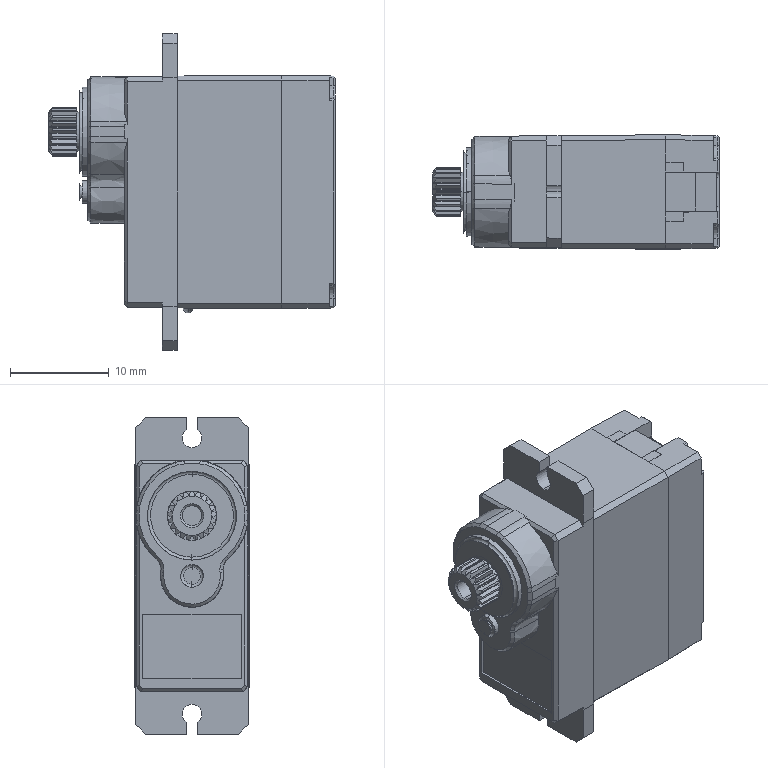Part | SolidWorks | 8 solids | 1094 faces | box 29 x 11.559 x 32.1 mm | volume 6256 mm3 | plane 441 | cylinder 418 | spline 112 | cone 91 | torus 32 | commonest cylinder face diameters 0.16 x66 0.1 x28 0.32 x24 7.8 x24 4.974 x22 0.08 x21